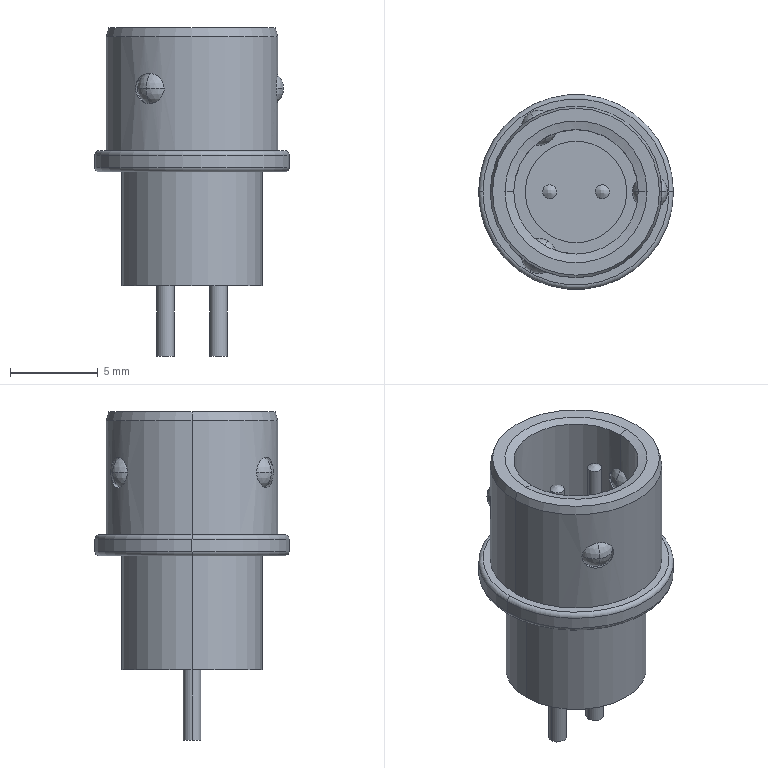Part | NX | features BREP 4 | 4 solids | 60 faces | box 11.1 x 11.1 x 18.7 mm | volume 715.454 mm3 | sphere 24 | cylinder 18 | plane 8 | torus 4 | cone 4 | spline 2 | commonest cylinder face diameters 0.8 x4 1 x4 5.783 x2 7.1 x2 8 x2 9.77 x2